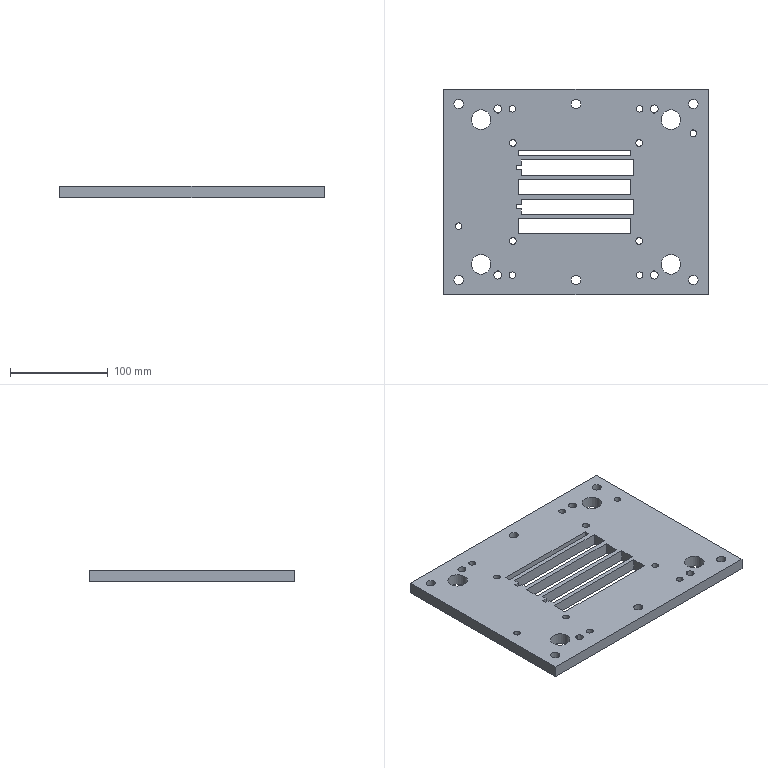Part | STEP file | 1 solid | 93 faces | box 270 x 210 x 12 mm | volume 556019 mm3 | cylinder 46 | plane 44 | cone 3 | commonest cylinder face diameters 1 x12 6.8 x10 11 x10 9.5 x6 8.01 x4 20 x4